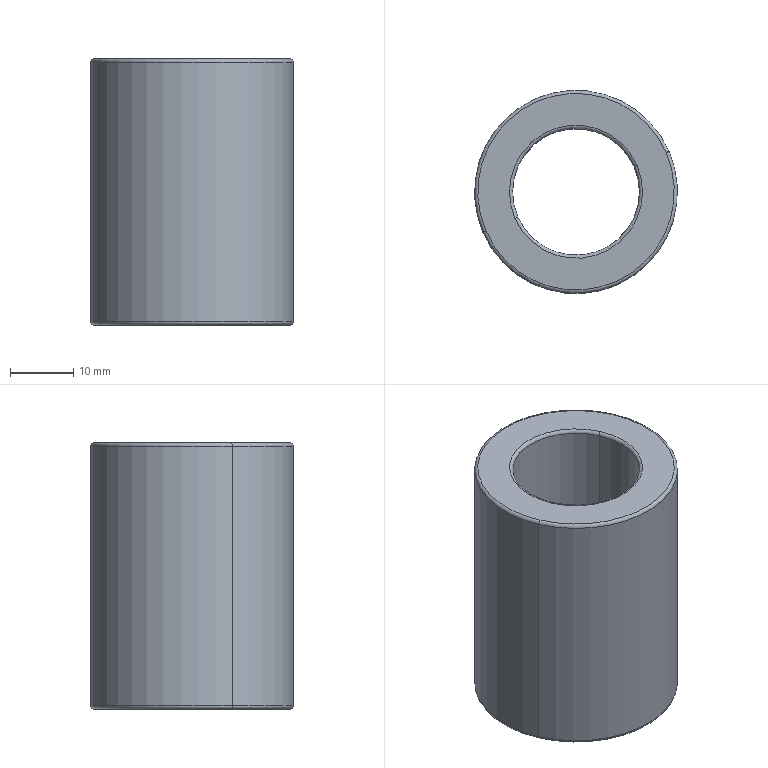Part | NX | features MISUMI__LMU-N200001 2 | 1 solid | 14 faces | box 32 x 32 x 42 mm | volume 20566 mm3 | torus 8 | cylinder 4 | plane 2 | commonest cylinder face diameters 20 x2 32 x2
STEP:
#1=CARTESIAN_POINT('',(-70.829,28.987,-327.629));
#2=VERTEX_POINT('',#1);
#3=CARTESIAN_POINT('',(-89.171,21.013,-327.629));
#4=VERTEX_POINT('',#3);
#5=CARTESIAN_POINT('',(-80.,25.,-327.629));
#6=DIRECTION('',(0.,0.,1.));
#7=DIRECTION('',(0.9171,0.3987,0.));
#8=AXIS2_PLACEMENT_3D('',#5,#6,#7);
#9=CIRCLE('',#8,10.);
#10=EDGE_CURVE('',#2,#4,#9,.T.);
#11=ORIENTED_EDGE('',*,*,#10,.T.);
#12=CARTESIAN_POINT('',(-89.629,20.813,-328.129));
#13=VERTEX_POINT('',#12);
#14=CARTESIAN_POINT('',(-89.629,20.813,-327.629));
#15=DIRECTION('',(0.3987,-0.9171,0.));
#16=DIRECTION('',(0.,0.,-1.));
#17=AXIS2_PLACEMENT_3D('',#14,#15,#16);
#18=CIRCLE('',#17,0.5);
#19=EDGE_CURVE('',#13,#4,#18,.T.);
#20=ORIENTED_EDGE('',*,*,#19,.F.);
#21=CARTESIAN_POINT('',(-70.371,29.187,-328.129));
#22=VERTEX_POINT('',#21);
#23=CARTESIAN_POINT('',(-80.,25.,-328.129));
#24=DIRECTION('',(0.,0.,1.));
#25=DIRECTION('',(0.9171,0.3987,0.));
#26=AXIS2_PLACEMENT_3D('',#23,#24,#25);
#27=CIRCLE('',#26,10.5);
#28=EDGE_CURVE('',#22,#13,#27,.T.);
#29=ORIENTED_EDGE('',*,*,#28,.F.);
#30=CARTESIAN_POINT('',(-70.371,29.187,-327.629));
#31=DIRECTION('',(-0.3987,0.9171,0.));
#32=DIRECTION('',(0.,0.,-1.));
#33=AXIS2_PLACEMENT_3D('',#30,#31,#32);
#34=CIRCLE('',#33,0.5);
#35=EDGE_CURVE('',#2,#22,#34,.F.);
#36=ORIENTED_EDGE('',*,*,#35,.F.);
#37=EDGE_LOOP('',(#11,#20,#29,#36));
#38=FACE_BOUND('',#37,.T.);
#39=CARTESIAN_POINT('',(-80.,25.,-327.629));
#40=DIRECTION('',(0.,0.,1.));
#41=DIRECTION('',(-0.9171,-0.3987,0.));
#42=AXIS2_PLACEMENT_3D('',#39,#40,#41);
#43=TOROIDAL_SURFACE('',#42,10.5,0.5);
#44=ADVANCED_FACE('',(#38),#43,.T.);
#45=CARTESIAN_POINT('',(-65.327,31.38,-286.629));
#46=VERTEX_POINT('',#45);
#47=CARTESIAN_POINT('',(-94.673,18.62,-286.629));
#48=VERTEX_POINT('',#47);
#49=CARTESIAN_POINT('',(-80.,25.,-286.629));
#50=DIRECTION('',(0.,0.,1.));
#51=DIRECTION('',(0.9171,0.3987,0.));
#52=AXIS2_PLACEMENT_3D('',#49,#50,#51);
#53=CIRCLE('',#52,16.);
#54=EDGE_CURVE('',#46,#48,#53,.T.);
#55=ORIENTED_EDGE('',*,*,#54,.T.);
#56=CARTESIAN_POINT('',(-94.215,18.82,-286.129));
#57=VERTEX_POINT('',#56);
#58=CARTESIAN_POINT('',(-94.215,18.82,-286.629));
#59=DIRECTION('',(0.3987,-0.9171,0.));
#60=DIRECTION('',(0.,0.,1.));
#61=AXIS2_PLACEMENT_3D('',#58,#59,#60);
#62=CIRCLE('',#61,0.5);
#63=EDGE_CURVE('',#57,#48,#62,.T.);
#64=ORIENTED_EDGE('',*,*,#63,.F.);
#65=CARTESIAN_POINT('',(-65.785,31.18,-286.129));
#66=VERTEX_POINT('',#65);
#67=CARTESIAN_POINT('',(-80.,25.,-286.129));
#68=DIRECTION('',(0.,0.,1.));
#69=DIRECTION('',(0.9171,0.3987,0.));
#70=AXIS2_PLACEMENT_3D('',#67,#68,#69);
#71=CIRCLE('',#70,15.5);
#72=EDGE_CURVE('',#66,#57,#71,.T.);
#73=ORIENTED_EDGE('',*,*,#72,.F.);
#74=CARTESIAN_POINT('',(-65.785,31.18,-286.629));
#75=DIRECTION('',(-0.3987,0.9171,0.));
#76=DIRECTION('',(0.,0.,1.));
#77=AXIS2_PLACEMENT_3D('',#74,#75,#76);
#78=CIRCLE('',#77,0.5);
#79=EDGE_CURVE('',#46,#66,#78,.F.);
#80=ORIENTED_EDGE('',*,*,#79,.F.);
#81=EDGE_LOOP('',(#55,#64,#73,#80));
#82=FACE_BOUND('',#81,.T.);
#83=CARTESIAN_POINT('',(-80.,25.,-286.629));
#84=DIRECTION('',(0.,0.,1.));
#85=DIRECTION('',(-0.9171,-0.3987,0.));
#86=AXIS2_PLACEMENT_3D('',#83,#84,#85);
#87=TOROIDAL_SURFACE('',#86,15.5,0.5);
#88=ADVANCED_FACE('',(#82),#87,.T.);
#89=CARTESIAN_POINT('',(-70.371,29.187,-286.129));
#90=VERTEX_POINT('',#89);
#91=CARTESIAN_POINT('',(-89.629,20.813,-286.129));
#92=VERTEX_POINT('',#91);
#93=CARTESIAN_POINT('',(-80.,25.,-286.129));
#94=DIRECTION('',(0.,0.,-1.));
#95=DIRECTION('',(0.9171,0.3987,0.));
#96=AXIS2_PLACEMENT_3D('',#93,#94,#95);
#97=CIRCLE('',#96,10.5);
#98=EDGE_CURVE('',#90,#92,#97,.T.);
#99=ORIENTED_EDGE('',*,*,#98,.T.);
#100=CARTESIAN_POINT('',(-80.,25.,-286.129));
#101=DIRECTION('',(0.,0.,-1.));
#102=DIRECTION('',(-0.9171,-0.3987,0.));
#103=AXIS2_PLACEMENT_3D('',#100,#101,#102);
#104=CIRCLE('',#103,10.5);
#105=EDGE_CURVE('',#92,#90,#104,.T.);
#106=ORIENTED_EDGE('',*,*,#105,.T.);
#107=EDGE_LOOP('',(#99,#106));
#108=FACE_BOUND('',#107,.T.);
#109=ORIENTED_EDGE('',*,*,#72,.T.);
#110=CARTESIAN_POINT('',(-80.,25.,-286.129));
#111=DIRECTION('',(0.,0.,1.));
#112=DIRECTION('',(-0.9171,-0.3987,0.));
#113=AXIS2_PLACEMENT_3D('',#110,#111,#112);
#114=CIRCLE('',#113,15.5);
#115=EDGE_CURVE('',#57,#66,#114,.T.);
#116=ORIENTED_EDGE('',*,*,#115,.T.);
#117=EDGE_LOOP('',(#109,#116));
#118=FACE_BOUND('',#117,.T.);
#119=CARTESIAN_POINT('',(-80.,25.,-286.129));
#120=DIRECTION('',(0.,0.,1.));
#121=DIRECTION('',(-0.9171,-0.3987,0.));
#122=AXIS2_PLACEMENT_3D('',#119,#120,#121);
#123=PLANE('',#122);
#124=ADVANCED_FACE('',(#108,#118),#123,.T.);
#125=CARTESIAN_POINT('',(-70.829,28.987,-286.629));
#126=VERTEX_POINT('',#125);
#127=CARTESIAN_POINT('',(-70.371,29.187,-286.629));
#128=DIRECTION('',(-0.3987,0.9171,0.));
#129=DIRECTION('',(-0.9171,-0.3987,0.));
#130=AXIS2_PLACEMENT_3D('',#127,#128,#129);
#131=CIRCLE('',#130,0.5);
#132=EDGE_CURVE('',#126,#90,#131,.T.);
#133=ORIENTED_EDGE('',*,*,#132,.F.);
#134=CARTESIAN_POINT('',(-89.171,21.013,-286.629));
#135=VERTEX_POINT('',#134);
#136=CARTESIAN_POINT('',(-80.,25.,-286.629));
#137=DIRECTION('',(0.,0.,-1.));
#138=DIRECTION('',(0.9171,0.3987,0.));
#139=AXIS2_PLACEMENT_3D('',#136,#137,#138);
#140=CIRCLE('',#139,10.);
#141=EDGE_CURVE('',#126,#135,#140,.T.);
#142=ORIENTED_EDGE('',*,*,#141,.T.);
#143=CARTESIAN_POINT('',(-89.629,20.813,-286.629));
#144=DIRECTION('',(0.3987,-0.9171,0.));
#145=DIRECTION('',(0.9171,0.3987,0.));
#146=AXIS2_PLACEMENT_3D('',#143,#144,#145);
#147=CIRCLE('',#146,0.5);
#148=EDGE_CURVE('',#92,#135,#147,.F.);
#149=ORIENTED_EDGE('',*,*,#148,.F.);
#150=ORIENTED_EDGE('',*,*,#98,.F.);
#151=EDGE_LOOP('',(#133,#142,#149,#150));
#152=FACE_BOUND('',#151,.T.);
#153=CARTESIAN_POINT('',(-80.,25.,-286.629));
#154=DIRECTION('',(0.,0.,1.));
#155=DIRECTION('',(-0.9171,-0.3987,0.));
#156=AXIS2_PLACEMENT_3D('',#153,#154,#155);
#157=TOROIDAL_SURFACE('',#156,10.5,0.5);
#158=ADVANCED_FACE('',(#152),#157,.T.);
#159=ORIENTED_EDGE('',*,*,#105,.F.);
#160=ORIENTED_EDGE('',*,*,#148,.T.);
#161=CARTESIAN_POINT('',(-80.,25.,-286.629));
#162=DIRECTION('',(0.,0.,-1.));
#163=DIRECTION('',(-0.9171,-0.3987,0.));
#164=AXIS2_PLACEMENT_3D('',#161,#162,#163);
#165=CIRCLE('',#164,10.);
#166=EDGE_CURVE('',#135,#126,#165,.T.);
#167=ORIENTED_EDGE('',*,*,#166,.T.);
#168=ORIENTED_EDGE('',*,*,#132,.T.);
#169=EDGE_LOOP('',(#159,#160,#167,#168));
#170=FACE_BOUND('',#169,.T.);
#171=CARTESIAN_POINT('',(-80.,25.,-286.629));
#172=DIRECTION('',(0.,0.,1.));
#173=DIRECTION('',(-0.9171,-0.3987,0.));
#174=AXIS2_PLACEMENT_3D('',#171,#172,#173);
#175=TOROIDAL_SURFACE('',#174,10.5,0.5);
#176=ADVANCED_FACE('',(#170),#175,.T.);
#177=CARTESIAN_POINT('',(-89.171,21.013,-327.629));
#178=DIRECTION('',(0.,0.,1.));
#179=VECTOR('',#178,1000.);
#180=LINE('',#177,#179);
#181=EDGE_CURVE('',#4,#135,#180,.T.);
#182=ORIENTED_EDGE('',*,*,#181,.F.);
#183=ORIENTED_EDGE('',*,*,#10,.F.);
#184=CARTESIAN_POINT('',(-70.829,28.987,-327.629));
#185=DIRECTION('',(0.,0.,1.));
#186=VECTOR('',#185,1000.);
#187=LINE('',#184,#186);
#188=EDGE_CURVE('',#126,#2,#187,.F.);
#189=ORIENTED_EDGE('',*,*,#188,.F.);
#190=ORIENTED_EDGE('',*,*,#166,.F.);
#191=EDGE_LOOP('',(#182,#183,#189,#190));
#192=FACE_BOUND('',#191,.T.);
#193=CARTESIAN_POINT('',(-80.,25.,-286.129));
#194=DIRECTION('',(0.,0.,-1.));
#195=DIRECTION('',(0.9171,0.3987,0.));
#196=AXIS2_PLACEMENT_3D('',#193,#194,#195);
#197=CYLINDRICAL_SURFACE('',#196,10.);
#198=ADVANCED_FACE('',(#192),#197,.F.);
#199=ORIENTED_EDGE('',*,*,#141,.F.);
#200=ORIENTED_EDGE('',*,*,#188,.T.);
#201=CARTESIAN_POINT('',(-80.,25.,-327.629));
#202=DIRECTION('',(0.,0.,1.));
#203=DIRECTION('',(-0.9171,-0.3987,0.));
#204=AXIS2_PLACEMENT_3D('',#201,#202,#203);
#205=CIRCLE('',#204,10.);
#206=EDGE_CURVE('',#4,#2,#205,.T.);
#207=ORIENTED_EDGE('',*,*,#206,.F.);
#208=ORIENTED_EDGE('',*,*,#181,.T.);
#209=EDGE_LOOP('',(#199,#200,#207,#208));
#210=FACE_BOUND('',#209,.T.);
#211=CARTESIAN_POINT('',(-80.,25.,-286.129));
#212=DIRECTION('',(0.,0.,-1.));
#213=DIRECTION('',(0.9171,0.3987,0.));
#214=AXIS2_PLACEMENT_3D('',#211,#212,#213);
#215=CYLINDRICAL_SURFACE('',#214,10.);
#216=ADVANCED_FACE('',(#210),#215,.F.);
#217=ORIENTED_EDGE('',*,*,#35,.T.);
#218=CARTESIAN_POINT('',(-80.,25.,-328.129));
#219=DIRECTION('',(0.,0.,1.));
#220=DIRECTION('',(-0.9171,-0.3987,0.));
#221=AXIS2_PLACEMENT_3D('',#218,#219,#220);
#222=CIRCLE('',#221,10.5);
#223=EDGE_CURVE('',#13,#22,#222,.T.);
#224=ORIENTED_EDGE('',*,*,#223,.F.);
#225=ORIENTED_EDGE('',*,*,#19,.T.);
#226=ORIENTED_EDGE('',*,*,#206,.T.);
#227=EDGE_LOOP('',(#217,#224,#225,#226));
#228=FACE_BOUND('',#227,.T.);
#229=CARTESIAN_POINT('',(-80.,25.,-327.629));
#230=DIRECTION('',(0.,0.,1.));
#231=DIRECTION('',(-0.9171,-0.3987,0.));
#232=AXIS2_PLACEMENT_3D('',#229,#230,#231);
#233=TOROIDAL_SURFACE('',#232,10.5,0.5);
#234=ADVANCED_FACE('',(#228),#233,.T.);
#235=ORIENTED_EDGE('',*,*,#28,.T.);
#236=ORIENTED_EDGE('',*,*,#223,.T.);
#237=EDGE_LOOP('',(#235,#236));
#238=FACE_BOUND('',#237,.T.);
#239=CARTESIAN_POINT('',(-65.785,31.18,-328.129));
#240=VERTEX_POINT('',#239);
#241=CARTESIAN_POINT('',(-94.215,18.82,-328.129));
#242=VERTEX_POINT('',#241);
#243=CARTESIAN_POINT('',(-80.,25.,-328.129));
#244=DIRECTION('',(0.,0.,-1.));
#245=DIRECTION('',(0.9171,0.3987,0.));
#246=AXIS2_PLACEMENT_3D('',#243,#244,#245);
#247=CIRCLE('',#246,15.5);
#248=EDGE_CURVE('',#240,#242,#247,.T.);
#249=ORIENTED_EDGE('',*,*,#248,.T.);
#250=CARTESIAN_POINT('',(-80.,25.,-328.129));
#251=DIRECTION('',(0.,0.,-1.));
#252=DIRECTION('',(-0.9171,-0.3987,0.));
#253=AXIS2_PLACEMENT_3D('',#250,#251,#252);
#254=CIRCLE('',#253,15.5);
#255=EDGE_CURVE('',#242,#240,#254,.T.);
#256=ORIENTED_EDGE('',*,*,#255,.T.);
#257=EDGE_LOOP('',(#249,#256));
#258=FACE_BOUND('',#257,.T.);
#259=CARTESIAN_POINT('',(-80.,25.,-328.129));
#260=DIRECTION('',(0.,0.,1.));
#261=DIRECTION('',(-0.9171,-0.3987,0.));
#262=AXIS2_PLACEMENT_3D('',#259,#260,#261);
#263=PLANE('',#262);
#264=ADVANCED_FACE('',(#238,#258),#263,.F.);
#265=CARTESIAN_POINT('',(-65.327,31.38,-327.629));
#266=VERTEX_POINT('',#265);
#267=CARTESIAN_POINT('',(-65.785,31.18,-327.629));
#268=DIRECTION('',(-0.3987,0.9171,0.));
#269=DIRECTION('',(0.9171,0.3987,0.));
#270=AXIS2_PLACEMENT_3D('',#267,#268,#269);
#271=CIRCLE('',#270,0.5);
#272=EDGE_CURVE('',#266,#240,#271,.T.);
#273=ORIENTED_EDGE('',*,*,#272,.F.);
#274=CARTESIAN_POINT('',(-94.673,18.62,-327.629));
#275=VERTEX_POINT('',#274);
#276=CARTESIAN_POINT('',(-80.,25.,-327.629));
#277=DIRECTION('',(0.,0.,-1.));
#278=DIRECTION('',(0.9171,0.3987,0.));
#279=AXIS2_PLACEMENT_3D('',#276,#277,#278);
#280=CIRCLE('',#279,16.);
#281=EDGE_CURVE('',#266,#275,#280,.T.);
#282=ORIENTED_EDGE('',*,*,#281,.T.);
#283=CARTESIAN_POINT('',(-94.215,18.82,-327.629));
#284=DIRECTION('',(0.3987,-0.9171,0.));
#285=DIRECTION('',(-0.9171,-0.3987,0.));
#286=AXIS2_PLACEMENT_3D('',#283,#284,#285);
#287=CIRCLE('',#286,0.5);
#288=EDGE_CURVE('',#242,#275,#287,.F.);
#289=ORIENTED_EDGE('',*,*,#288,.F.);
#290=ORIENTED_EDGE('',*,*,#248,.F.);
#291=EDGE_LOOP('',(#273,#282,#289,#290));
#292=FACE_BOUND('',#291,.T.);
#293=CARTESIAN_POINT('',(-80.,25.,-327.629));
#294=DIRECTION('',(0.,0.,1.));
#295=DIRECTION('',(-0.9171,-0.3987,0.));
#296=AXIS2_PLACEMENT_3D('',#293,#294,#295);
#297=TOROIDAL_SURFACE('',#296,15.5,0.5);
#298=ADVANCED_FACE('',(#292),#297,.T.);
#299=ORIENTED_EDGE('',*,*,#255,.F.);
#300=ORIENTED_EDGE('',*,*,#288,.T.);
#301=CARTESIAN_POINT('',(-80.,25.,-327.629));
#302=DIRECTION('',(0.,0.,-1.));
#303=DIRECTION('',(-0.9171,-0.3987,0.));
#304=AXIS2_PLACEMENT_3D('',#301,#302,#303);
#305=CIRCLE('',#304,16.);
#306=EDGE_CURVE('',#275,#266,#305,.T.);
#307=ORIENTED_EDGE('',*,*,#306,.T.);
#308=ORIENTED_EDGE('',*,*,#272,.T.);
#309=EDGE_LOOP('',(#299,#300,#307,#308));
#310=FACE_BOUND('',#309,.T.);
#311=CARTESIAN_POINT('',(-80.,25.,-327.629));
#312=DIRECTION('',(0.,0.,1.));
#313=DIRECTION('',(-0.9171,-0.3987,0.));
#314=AXIS2_PLACEMENT_3D('',#311,#312,#313);
#315=TOROIDAL_SURFACE('',#314,15.5,0.5);
#316=ADVANCED_FACE('',(#310),#315,.T.);
#317=ORIENTED_EDGE('',*,*,#54,.F.);
#318=CARTESIAN_POINT('',(-65.327,31.38,-327.629));
#319=DIRECTION('',(0.,0.,1.));
#320=VECTOR('',#319,1000.);
#321=LINE('',#318,#320);
#322=EDGE_CURVE('',#266,#46,#321,.T.);
#323=ORIENTED_EDGE('',*,*,#322,.F.);
#324=ORIENTED_EDGE('',*,*,#306,.F.);
#325=CARTESIAN_POINT('',(-94.673,18.62,-327.629));
#326=DIRECTION('',(0.,0.,1.));
#327=VECTOR('',#326,1000.);
#328=LINE('',#325,#327);
#329=EDGE_CURVE('',#48,#275,#328,.F.);
#330=ORIENTED_EDGE('',*,*,#329,.F.);
#331=EDGE_LOOP('',(#317,#323,#324,#330));
#332=FACE_BOUND('',#331,.T.);
#333=CARTESIAN_POINT('',(-80.,25.,-286.129));
#334=DIRECTION('',(0.,0.,-1.));
#335=DIRECTION('',(0.9171,0.3987,0.));
#336=AXIS2_PLACEMENT_3D('',#333,#334,#335);
#337=CYLINDRICAL_SURFACE('',#336,16.);
#338=ADVANCED_FACE('',(#332),#337,.T.);
#339=ORIENTED_EDGE('',*,*,#329,.T.);
#340=ORIENTED_EDGE('',*,*,#281,.F.);
#341=ORIENTED_EDGE('',*,*,#322,.T.);
#342=CARTESIAN_POINT('',(-80.,25.,-286.629));
#343=DIRECTION('',(0.,0.,1.));
#344=DIRECTION('',(-0.9171,-0.3987,0.));
#345=AXIS2_PLACEMENT_3D('',#342,#343,#344);
#346=CIRCLE('',#345,16.);
#347=EDGE_CURVE('',#48,#46,#346,.T.);
#348=ORIENTED_EDGE('',*,*,#347,.F.);
#349=EDGE_LOOP('',(#339,#340,#341,#348));
#350=FACE_BOUND('',#349,.T.);
#351=CARTESIAN_POINT('',(-80.,25.,-286.129));
#352=DIRECTION('',(0.,0.,-1.));
#353=DIRECTION('',(0.9171,0.3987,0.));
#354=AXIS2_PLACEMENT_3D('',#351,#352,#353);
#355=CYLINDRICAL_SURFACE('',#354,16.);
#356=ADVANCED_FACE('',(#350),#355,.T.);
#357=ORIENTED_EDGE('',*,*,#79,.T.);
#358=ORIENTED_EDGE('',*,*,#115,.F.);
#359=ORIENTED_EDGE('',*,*,#63,.T.);
#360=ORIENTED_EDGE('',*,*,#347,.T.);
#361=EDGE_LOOP('',(#357,#358,#359,#360));
#362=FACE_BOUND('',#361,.T.);
#363=CARTESIAN_POINT('',(-80.,25.,-286.629));
#364=DIRECTION('',(0.,0.,1.));
#365=DIRECTION('',(-0.9171,-0.3987,0.));
#366=AXIS2_PLACEMENT_3D('',#363,#364,#365);
#367=TOROIDAL_SURFACE('',#366,15.5,0.5);
#368=ADVANCED_FACE('',(#362),#367,.T.);
#369=CLOSED_SHELL('',(#44,#88,#124,#158,#176,#198,#216,#234,#264,#298,#316,#338,#356,#368));
#370=MANIFOLD_SOLID_BREP('',#369);
#371=(LENGTH_UNIT()NAMED_UNIT(*)SI_UNIT(.MILLI.,.METRE.));
#372=UNCERTAINTY_MEASURE_WITH_UNIT(LENGTH_MEASURE(0.00001),#371,'','');
#373=(NAMED_UNIT(*)PLANE_ANGLE_UNIT()SI_UNIT($,.RADIAN.));
#374=(NAMED_UNIT(*)SI_UNIT($,.STERADIAN.)SOLID_ANGLE_UNIT());
#375=(GEOMETRIC_REPRESENTATION_CONTEXT(3)GLOBAL_UNCERTAINTY_ASSIGNED_CONTEXT((#372))GLOBAL_UNIT_ASSIGNED_CONTEXT((#371,#373,#374))REPRESENTATION_CONTEXT('',''));
#376=ADVANCED_BREP_SHAPE_REPRESENTATION('',(#370),#375);